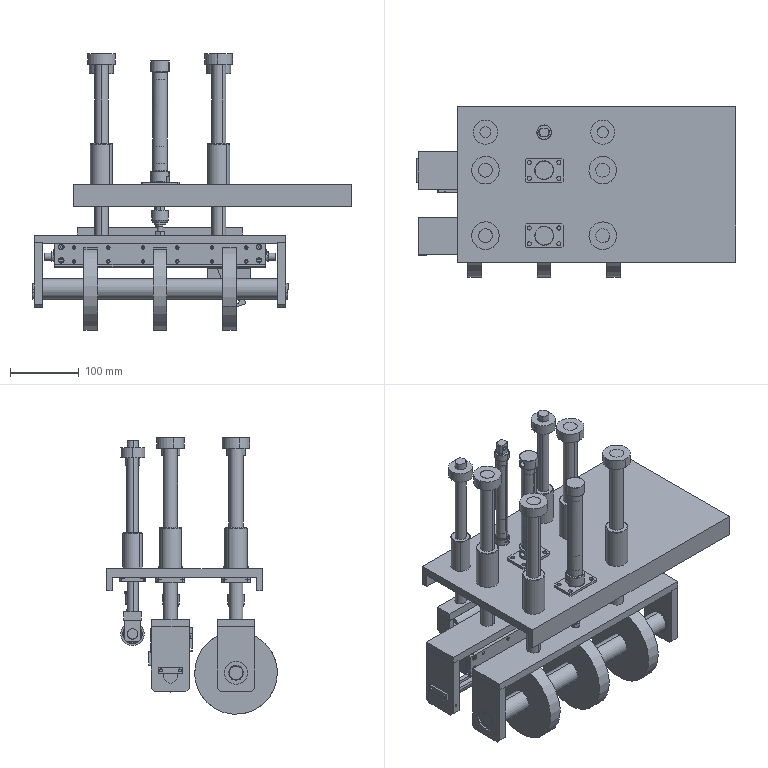Part | SolidWorks | features MirrorCompFeat 1 | 67 solids | 2132 faces | box 463.5 x 247.5 x 400.75 mm | volume 4348981 mm3 | plane 988 | cylinder 759 | cone 305 | spline 80 | commonest cylinder face diameters 20 x51 4.134 x40 4.5 x36 9 x36 5.5 x34 6 x32